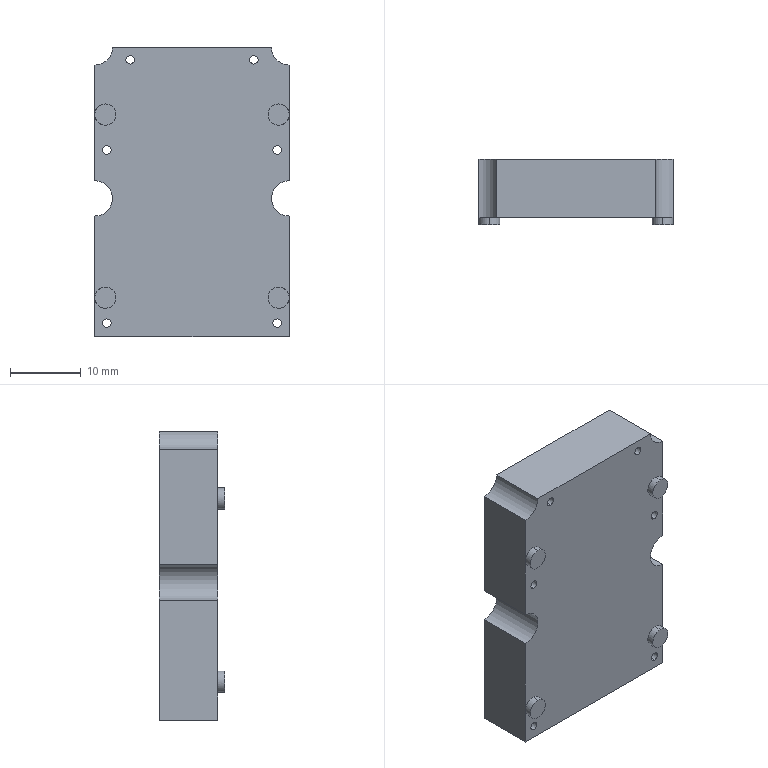Part | SolidWorks | features Extrusion 1, ICE 1, Scale 1 | 1 solid | 36 faces | box 27.5 x 9.25 x 40.9 mm | volume 9008 mm3 | cylinder 24 | plane 12 | commonest cylinder face diameters 1.2 x12 3 x8 5 x4
STEP:
#1=CARTESIAN_POINT('',(-12.25,3.11,-16.627));
#2=VERTEX_POINT('',#1);
#3=CARTESIAN_POINT('',(-12.25,3.11,-13.627));
#4=VERTEX_POINT('',#3);
#5=CARTESIAN_POINT('',(-12.25,3.11,-15.127));
#6=DIRECTION('',(0.,-1.,0.));
#7=DIRECTION('',(0.,0.,-1.));
#8=AXIS2_PLACEMENT_3D('',#5,#6,#7);
#9=CIRCLE('',#8,1.5);
#10=EDGE_CURVE('',#2,#4,#9,.T.);
#11=ORIENTED_EDGE('',*,*,#10,.F.);
#12=CARTESIAN_POINT('',(-12.25,4.11,-16.627));
#13=VERTEX_POINT('',#12);
#14=CARTESIAN_POINT('',(-12.25,3.11,-16.627));
#15=DIRECTION('',(0.,1.,0.));
#16=VECTOR('',#15,1000.);
#17=LINE('',#14,#16);
#18=EDGE_CURVE('',#2,#13,#17,.T.);
#19=ORIENTED_EDGE('',*,*,#18,.T.);
#20=CARTESIAN_POINT('',(-12.25,4.11,-13.627));
#21=VERTEX_POINT('',#20);
#22=CARTESIAN_POINT('',(-12.25,4.11,-15.127));
#23=DIRECTION('',(0.,-1.,0.));
#24=DIRECTION('',(0.,0.,-1.));
#25=AXIS2_PLACEMENT_3D('',#22,#23,#24);
#26=CIRCLE('',#25,1.5);
#27=EDGE_CURVE('',#13,#21,#26,.T.);
#28=ORIENTED_EDGE('',*,*,#27,.T.);
#29=CARTESIAN_POINT('',(-12.25,3.11,-13.627));
#30=DIRECTION('',(0.,1.,0.));
#31=VECTOR('',#30,1000.);
#32=LINE('',#29,#31);
#33=EDGE_CURVE('',#4,#21,#32,.T.);
#34=ORIENTED_EDGE('',*,*,#33,.F.);
#35=EDGE_LOOP('',(#11,#19,#28,#34));
#36=FACE_OUTER_BOUND('',#35,.T.);
#37=CARTESIAN_POINT('',(-12.25,3.11,-15.127));
#38=DIRECTION('',(0.,1.,0.));
#39=DIRECTION('',(0.,0.,1.));
#40=AXIS2_PLACEMENT_3D('',#37,#38,#39);
#41=CYLINDRICAL_SURFACE('',#40,1.5);
#42=ADVANCED_FACE('',(#36),#41,.T.);
#43=CARTESIAN_POINT('',(-12.25,3.11,9.273));
#44=VERTEX_POINT('',#43);
#45=CARTESIAN_POINT('',(-12.25,3.11,12.273));
#46=VERTEX_POINT('',#45);
#47=CARTESIAN_POINT('',(-12.25,3.11,10.773));
#48=DIRECTION('',(0.,-1.,0.));
#49=DIRECTION('',(0.,0.,-1.));
#50=AXIS2_PLACEMENT_3D('',#47,#48,#49);
#51=CIRCLE('',#50,1.5);
#52=EDGE_CURVE('',#44,#46,#51,.T.);
#53=ORIENTED_EDGE('',*,*,#52,.F.);
#54=CARTESIAN_POINT('',(-12.25,4.11,9.273));
#55=VERTEX_POINT('',#54);
#56=CARTESIAN_POINT('',(-12.25,3.11,9.273));
#57=DIRECTION('',(0.,1.,0.));
#58=VECTOR('',#57,1000.);
#59=LINE('',#56,#58);
#60=EDGE_CURVE('',#44,#55,#59,.T.);
#61=ORIENTED_EDGE('',*,*,#60,.T.);
#62=CARTESIAN_POINT('',(-12.25,4.11,12.273));
#63=VERTEX_POINT('',#62);
#64=CARTESIAN_POINT('',(-12.25,4.11,10.773));
#65=DIRECTION('',(0.,-1.,0.));
#66=DIRECTION('',(0.,0.,-1.));
#67=AXIS2_PLACEMENT_3D('',#64,#65,#66);
#68=CIRCLE('',#67,1.5);
#69=EDGE_CURVE('',#55,#63,#68,.T.);
#70=ORIENTED_EDGE('',*,*,#69,.T.);
#71=CARTESIAN_POINT('',(-12.25,3.11,12.273));
#72=DIRECTION('',(0.,1.,0.));
#73=VECTOR('',#72,1000.);
#74=LINE('',#71,#73);
#75=EDGE_CURVE('',#46,#63,#74,.T.);
#76=ORIENTED_EDGE('',*,*,#75,.F.);
#77=EDGE_LOOP('',(#53,#61,#70,#76));
#78=FACE_OUTER_BOUND('',#77,.T.);
#79=CARTESIAN_POINT('',(-12.25,3.11,10.773));
#80=DIRECTION('',(0.,1.,0.));
#81=DIRECTION('',(0.,0.,1.));
#82=AXIS2_PLACEMENT_3D('',#79,#80,#81);
#83=CYLINDRICAL_SURFACE('',#82,1.5);
#84=ADVANCED_FACE('',(#78),#83,.T.);
#85=CARTESIAN_POINT('',(12.25,3.11,9.273));
#86=VERTEX_POINT('',#85);
#87=CARTESIAN_POINT('',(12.25,3.11,12.273));
#88=VERTEX_POINT('',#87);
#89=CARTESIAN_POINT('',(12.25,3.11,10.773));
#90=DIRECTION('',(0.,-1.,0.));
#91=DIRECTION('',(0.,0.,-1.));
#92=AXIS2_PLACEMENT_3D('',#89,#90,#91);
#93=CIRCLE('',#92,1.5);
#94=EDGE_CURVE('',#86,#88,#93,.T.);
#95=ORIENTED_EDGE('',*,*,#94,.F.);
#96=CARTESIAN_POINT('',(12.25,4.11,9.273));
#97=VERTEX_POINT('',#96);
#98=CARTESIAN_POINT('',(12.25,3.11,9.273));
#99=DIRECTION('',(0.,1.,0.));
#100=VECTOR('',#99,1000.);
#101=LINE('',#98,#100);
#102=EDGE_CURVE('',#86,#97,#101,.T.);
#103=ORIENTED_EDGE('',*,*,#102,.T.);
#104=CARTESIAN_POINT('',(13.75,4.11,10.773));
#105=VERTEX_POINT('',#104);
#106=CARTESIAN_POINT('',(12.25,4.11,10.773));
#107=DIRECTION('',(0.,-1.,0.));
#108=DIRECTION('',(0.,0.,-1.));
#109=AXIS2_PLACEMENT_3D('',#106,#107,#108);
#110=CIRCLE('',#109,1.5);
#111=EDGE_CURVE('',#97,#105,#110,.T.);
#112=ORIENTED_EDGE('',*,*,#111,.T.);
#113=CARTESIAN_POINT('',(12.25,4.11,12.273));
#114=VERTEX_POINT('',#113);
#115=CARTESIAN_POINT('',(12.25,4.11,10.773));
#116=DIRECTION('',(0.,-1.,0.));
#117=DIRECTION('',(0.,0.,-1.));
#118=AXIS2_PLACEMENT_3D('',#115,#116,#117);
#119=CIRCLE('',#118,1.5);
#120=EDGE_CURVE('',#105,#114,#119,.T.);
#121=ORIENTED_EDGE('',*,*,#120,.T.);
#122=CARTESIAN_POINT('',(12.25,3.11,12.273));
#123=DIRECTION('',(0.,1.,0.));
#124=VECTOR('',#123,1000.);
#125=LINE('',#122,#124);
#126=EDGE_CURVE('',#88,#114,#125,.T.);
#127=ORIENTED_EDGE('',*,*,#126,.F.);
#128=EDGE_LOOP('',(#95,#103,#112,#121,#127));
#129=FACE_OUTER_BOUND('',#128,.T.);
#130=CARTESIAN_POINT('',(12.25,3.11,10.773));
#131=DIRECTION('',(0.,1.,0.));
#132=DIRECTION('',(0.,0.,1.));
#133=AXIS2_PLACEMENT_3D('',#130,#131,#132);
#134=CYLINDRICAL_SURFACE('',#133,1.5);
#135=ADVANCED_FACE('',(#129),#134,.T.);
#136=CARTESIAN_POINT('',(12.25,3.11,-16.627));
#137=VERTEX_POINT('',#136);
#138=CARTESIAN_POINT('',(12.25,3.11,-13.627));
#139=VERTEX_POINT('',#138);
#140=CARTESIAN_POINT('',(12.25,3.11,-15.127));
#141=DIRECTION('',(0.,-1.,0.));
#142=DIRECTION('',(0.,0.,-1.));
#143=AXIS2_PLACEMENT_3D('',#140,#141,#142);
#144=CIRCLE('',#143,1.5);
#145=EDGE_CURVE('',#137,#139,#144,.T.);
#146=ORIENTED_EDGE('',*,*,#145,.F.);
#147=CARTESIAN_POINT('',(12.25,4.11,-16.627));
#148=VERTEX_POINT('',#147);
#149=CARTESIAN_POINT('',(12.25,3.11,-16.627));
#150=DIRECTION('',(0.,1.,0.));
#151=VECTOR('',#150,1000.);
#152=LINE('',#149,#151);
#153=EDGE_CURVE('',#137,#148,#152,.T.);
#154=ORIENTED_EDGE('',*,*,#153,.T.);
#155=CARTESIAN_POINT('',(13.75,4.11,-15.127));
#156=VERTEX_POINT('',#155);
#157=CARTESIAN_POINT('',(12.25,4.11,-15.127));
#158=DIRECTION('',(0.,-1.,0.));
#159=DIRECTION('',(0.,0.,-1.));
#160=AXIS2_PLACEMENT_3D('',#157,#158,#159);
#161=CIRCLE('',#160,1.5);
#162=EDGE_CURVE('',#148,#156,#161,.T.);
#163=ORIENTED_EDGE('',*,*,#162,.T.);
#164=CARTESIAN_POINT('',(12.25,4.11,-13.627));
#165=VERTEX_POINT('',#164);
#166=CARTESIAN_POINT('',(12.25,4.11,-15.127));
#167=DIRECTION('',(0.,-1.,0.));
#168=DIRECTION('',(0.,0.,-1.));
#169=AXIS2_PLACEMENT_3D('',#166,#167,#168);
#170=CIRCLE('',#169,1.5);
#171=EDGE_CURVE('',#156,#165,#170,.T.);
#172=ORIENTED_EDGE('',*,*,#171,.T.);
#173=CARTESIAN_POINT('',(12.25,3.11,-13.627));
#174=DIRECTION('',(0.,1.,0.));
#175=VECTOR('',#174,1000.);
#176=LINE('',#173,#175);
#177=EDGE_CURVE('',#139,#165,#176,.T.);
#178=ORIENTED_EDGE('',*,*,#177,.F.);
#179=EDGE_LOOP('',(#146,#154,#163,#172,#178));
#180=FACE_OUTER_BOUND('',#179,.T.);
#181=CARTESIAN_POINT('',(12.25,3.11,-15.127));
#182=DIRECTION('',(0.,1.,0.));
#183=DIRECTION('',(0.,0.,1.));
#184=AXIS2_PLACEMENT_3D('',#181,#182,#183);
#185=CYLINDRICAL_SURFACE('',#184,1.5);
#186=ADVANCED_FACE('',(#180),#185,.T.);
#187=CARTESIAN_POINT('',(12.05,12.36,-19.327));
#188=VERTEX_POINT('',#187);
#189=CARTESIAN_POINT('',(12.05,12.36,-18.127));
#190=VERTEX_POINT('',#189);
#191=CARTESIAN_POINT('',(12.05,12.36,-18.727));
#192=DIRECTION('',(0.,1.,0.));
#193=DIRECTION('',(0.,0.,-1.));
#194=AXIS2_PLACEMENT_3D('',#191,#192,#193);
#195=CIRCLE('',#194,0.6);
#196=EDGE_CURVE('',#188,#190,#195,.T.);
#197=ORIENTED_EDGE('',*,*,#196,.T.);
#198=CARTESIAN_POINT('',(12.05,4.11,-18.127));
#199=VERTEX_POINT('',#198);
#200=CARTESIAN_POINT('',(12.05,12.36,-18.127));
#201=DIRECTION('',(0.,-1.,0.));
#202=VECTOR('',#201,1000.);
#203=LINE('',#200,#202);
#204=EDGE_CURVE('',#190,#199,#203,.T.);
#205=ORIENTED_EDGE('',*,*,#204,.T.);
#206=CARTESIAN_POINT('',(12.05,4.11,-19.327));
#207=VERTEX_POINT('',#206);
#208=CARTESIAN_POINT('',(12.05,4.11,-18.727));
#209=DIRECTION('',(0.,1.,0.));
#210=DIRECTION('',(0.,0.,-1.));
#211=AXIS2_PLACEMENT_3D('',#208,#209,#210);
#212=CIRCLE('',#211,0.6);
#213=EDGE_CURVE('',#207,#199,#212,.T.);
#214=ORIENTED_EDGE('',*,*,#213,.F.);
#215=CARTESIAN_POINT('',(12.05,12.36,-19.327));
#216=DIRECTION('',(0.,-1.,0.));
#217=VECTOR('',#216,1000.);
#218=LINE('',#215,#217);
#219=EDGE_CURVE('',#188,#207,#218,.T.);
#220=ORIENTED_EDGE('',*,*,#219,.F.);
#221=EDGE_LOOP('',(#197,#205,#214,#220));
#222=FACE_OUTER_BOUND('',#221,.T.);
#223=CARTESIAN_POINT('',(12.05,12.36,-18.727));
#224=DIRECTION('',(0.,-1.,0.));
#225=DIRECTION('',(0.,0.,-1.));
#226=AXIS2_PLACEMENT_3D('',#223,#224,#225);
#227=CYLINDRICAL_SURFACE('',#226,0.6);
#228=ADVANCED_FACE('',(#222),#227,.F.);
#229=CARTESIAN_POINT('',(12.05,12.36,5.173));
#230=VERTEX_POINT('',#229);
#231=CARTESIAN_POINT('',(12.05,12.36,6.373));
#232=VERTEX_POINT('',#231);
#233=CARTESIAN_POINT('',(12.05,12.36,5.773));
#234=DIRECTION('',(0.,1.,0.));
#235=DIRECTION('',(0.,0.,-1.));
#236=AXIS2_PLACEMENT_3D('',#233,#234,#235);
#237=CIRCLE('',#236,0.6);
#238=EDGE_CURVE('',#230,#232,#237,.T.);
#239=ORIENTED_EDGE('',*,*,#238,.T.);
#240=CARTESIAN_POINT('',(12.05,4.11,6.373));
#241=VERTEX_POINT('',#240);
#242=CARTESIAN_POINT('',(12.05,12.36,6.373));
#243=DIRECTION('',(0.,-1.,0.));
#244=VECTOR('',#243,1000.);
#245=LINE('',#242,#244);
#246=EDGE_CURVE('',#232,#241,#245,.T.);
#247=ORIENTED_EDGE('',*,*,#246,.T.);
#248=CARTESIAN_POINT('',(12.05,4.11,5.173));
#249=VERTEX_POINT('',#248);
#250=CARTESIAN_POINT('',(12.05,4.11,5.773));
#251=DIRECTION('',(0.,1.,0.));
#252=DIRECTION('',(0.,0.,-1.));
#253=AXIS2_PLACEMENT_3D('',#250,#251,#252);
#254=CIRCLE('',#253,0.6);
#255=EDGE_CURVE('',#249,#241,#254,.T.);
#256=ORIENTED_EDGE('',*,*,#255,.F.);
#257=CARTESIAN_POINT('',(12.05,12.36,5.173));
#258=DIRECTION('',(0.,-1.,0.));
#259=VECTOR('',#258,1000.);
#260=LINE('',#257,#259);
#261=EDGE_CURVE('',#230,#249,#260,.T.);
#262=ORIENTED_EDGE('',*,*,#261,.F.);
#263=EDGE_LOOP('',(#239,#247,#256,#262));
#264=FACE_OUTER_BOUND('',#263,.T.);
#265=CARTESIAN_POINT('',(12.05,12.36,5.773));
#266=DIRECTION('',(0.,-1.,0.));
#267=DIRECTION('',(0.,0.,-1.));
#268=AXIS2_PLACEMENT_3D('',#265,#266,#267);
#269=CYLINDRICAL_SURFACE('',#268,0.6);
#270=ADVANCED_FACE('',(#264),#269,.F.);
#271=CARTESIAN_POINT('',(8.75,12.36,17.923));
#272=VERTEX_POINT('',#271);
#273=CARTESIAN_POINT('',(8.75,12.36,19.123));
#274=VERTEX_POINT('',#273);
#275=CARTESIAN_POINT('',(8.75,12.36,18.523));
#276=DIRECTION('',(0.,1.,0.));
#277=DIRECTION('',(0.,0.,-1.));
#278=AXIS2_PLACEMENT_3D('',#275,#276,#277);
#279=CIRCLE('',#278,0.6);
#280=EDGE_CURVE('',#272,#274,#279,.T.);
#281=ORIENTED_EDGE('',*,*,#280,.T.);
#282=CARTESIAN_POINT('',(8.75,4.11,19.123));
#283=VERTEX_POINT('',#282);
#284=CARTESIAN_POINT('',(8.75,12.36,19.123));
#285=DIRECTION('',(0.,-1.,0.));
#286=VECTOR('',#285,1000.);
#287=LINE('',#284,#286);
#288=EDGE_CURVE('',#274,#283,#287,.T.);
#289=ORIENTED_EDGE('',*,*,#288,.T.);
#290=CARTESIAN_POINT('',(8.75,4.11,17.923));
#291=VERTEX_POINT('',#290);
#292=CARTESIAN_POINT('',(8.75,4.11,18.523));
#293=DIRECTION('',(0.,1.,0.));
#294=DIRECTION('',(0.,0.,-1.));
#295=AXIS2_PLACEMENT_3D('',#292,#293,#294);
#296=CIRCLE('',#295,0.6);
#297=EDGE_CURVE('',#291,#283,#296,.T.);
#298=ORIENTED_EDGE('',*,*,#297,.F.);
#299=CARTESIAN_POINT('',(8.75,12.36,17.923));
#300=DIRECTION('',(0.,-1.,0.));
#301=VECTOR('',#300,1000.);
#302=LINE('',#299,#301);
#303=EDGE_CURVE('',#272,#291,#302,.T.);
#304=ORIENTED_EDGE('',*,*,#303,.F.);
#305=EDGE_LOOP('',(#281,#289,#298,#304));
#306=FACE_OUTER_BOUND('',#305,.T.);
#307=CARTESIAN_POINT('',(8.75,12.36,18.523));
#308=DIRECTION('',(0.,-1.,0.));
#309=DIRECTION('',(0.,0.,-1.));
#310=AXIS2_PLACEMENT_3D('',#307,#308,#309);
#311=CYLINDRICAL_SURFACE('',#310,0.6);
#312=ADVANCED_FACE('',(#306),#311,.F.);
#313=CARTESIAN_POINT('',(-8.75,12.36,17.923));
#314=VERTEX_POINT('',#313);
#315=CARTESIAN_POINT('',(-8.75,12.36,19.123));
#316=VERTEX_POINT('',#315);
#317=CARTESIAN_POINT('',(-8.75,12.36,18.523));
#318=DIRECTION('',(0.,1.,0.));
#319=DIRECTION('',(0.,0.,1.));
#320=AXIS2_PLACEMENT_3D('',#317,#318,#319);
#321=CIRCLE('',#320,0.6);
#322=EDGE_CURVE('',#314,#316,#321,.T.);
#323=ORIENTED_EDGE('',*,*,#322,.T.);
#324=CARTESIAN_POINT('',(-8.75,4.11,19.123));
#325=VERTEX_POINT('',#324);
#326=CARTESIAN_POINT('',(-8.75,12.36,19.123));
#327=DIRECTION('',(0.,-1.,0.));
#328=VECTOR('',#327,1000.);
#329=LINE('',#326,#328);
#330=EDGE_CURVE('',#316,#325,#329,.T.);
#331=ORIENTED_EDGE('',*,*,#330,.T.);
#332=CARTESIAN_POINT('',(-8.75,4.11,17.923));
#333=VERTEX_POINT('',#332);
#334=CARTESIAN_POINT('',(-8.75,4.11,18.523));
#335=DIRECTION('',(0.,1.,0.));
#336=DIRECTION('',(0.,0.,1.));
#337=AXIS2_PLACEMENT_3D('',#334,#335,#336);
#338=CIRCLE('',#337,0.6);
#339=EDGE_CURVE('',#333,#325,#338,.T.);
#340=ORIENTED_EDGE('',*,*,#339,.F.);
#341=CARTESIAN_POINT('',(-8.75,12.36,17.923));
#342=DIRECTION('',(0.,-1.,0.));
#343=VECTOR('',#342,1000.);
#344=LINE('',#341,#343);
#345=EDGE_CURVE('',#314,#333,#344,.T.);
#346=ORIENTED_EDGE('',*,*,#345,.F.);
#347=EDGE_LOOP('',(#323,#331,#340,#346));
#348=FACE_OUTER_BOUND('',#347,.T.);
#349=CARTESIAN_POINT('',(-8.75,12.36,18.523));
#350=DIRECTION('',(0.,-1.,0.));
#351=DIRECTION('',(0.,0.,-1.));
#352=AXIS2_PLACEMENT_3D('',#349,#350,#351);
#353=CYLINDRICAL_SURFACE('',#352,0.6);
#354=ADVANCED_FACE('',(#348),#353,.F.);
#355=CARTESIAN_POINT('',(-12.05,12.36,5.173));
#356=VERTEX_POINT('',#355);
#357=CARTESIAN_POINT('',(-12.05,12.36,6.373));
#358=VERTEX_POINT('',#357);
#359=CARTESIAN_POINT('',(-12.05,12.36,5.773));
#360=DIRECTION('',(0.,1.,0.));
#361=DIRECTION('',(0.,0.,1.));
#362=AXIS2_PLACEMENT_3D('',#359,#360,#361);
#363=CIRCLE('',#362,0.6);
#364=EDGE_CURVE('',#356,#358,#363,.T.);
#365=ORIENTED_EDGE('',*,*,#364,.T.);
#366=CARTESIAN_POINT('',(-12.05,4.11,6.373));
#367=VERTEX_POINT('',#366);
#368=CARTESIAN_POINT('',(-12.05,12.36,6.373));
#369=DIRECTION('',(0.,-1.,0.));
#370=VECTOR('',#369,1000.);
#371=LINE('',#368,#370);
#372=EDGE_CURVE('',#358,#367,#371,.T.);
#373=ORIENTED_EDGE('',*,*,#372,.T.);
#374=CARTESIAN_POINT('',(-12.05,4.11,5.173));
#375=VERTEX_POINT('',#374);
#376=CARTESIAN_POINT('',(-12.05,4.11,5.773));
#377=DIRECTION('',(0.,1.,0.));
#378=DIRECTION('',(0.,0.,1.));
#379=AXIS2_PLACEMENT_3D('',#376,#377,#378);
#380=CIRCLE('',#379,0.6);
#381=EDGE_CURVE('',#375,#367,#380,.T.);
#382=ORIENTED_EDGE('',*,*,#381,.F.);
#383=CARTESIAN_POINT('',(-12.05,12.36,5.173));
#384=DIRECTION('',(0.,-1.,0.));
#385=VECTOR('',#384,1000.);
#386=LINE('',#383,#385);
#387=EDGE_CURVE('',#356,#375,#386,.T.);
#388=ORIENTED_EDGE('',*,*,#387,.F.);
#389=EDGE_LOOP('',(#365,#373,#382,#388));
#390=FACE_OUTER_BOUND('',#389,.T.);
#391=CARTESIAN_POINT('',(-12.05,12.36,5.773));
#392=DIRECTION('',(0.,-1.,0.));
#393=DIRECTION('',(0.,0.,-1.));
#394=AXIS2_PLACEMENT_3D('',#391,#392,#393);
#395=CYLINDRICAL_SURFACE('',#394,0.6);
#396=ADVANCED_FACE('',(#390),#395,.F.);
#397=CARTESIAN_POINT('',(-12.05,12.36,-19.327));
#398=VERTEX_POINT('',#397);
#399=CARTESIAN_POINT('',(-12.05,12.36,-18.127));
#400=VERTEX_POINT('',#399);
#401=CARTESIAN_POINT('',(-12.05,12.36,-18.727));
#402=DIRECTION('',(0.,1.,0.));
#403=DIRECTION('',(0.,0.,1.));
#404=AXIS2_PLACEMENT_3D('',#401,#402,#403);
#405=CIRCLE('',#404,0.6);
#406=EDGE_CURVE('',#398,#400,#405,.T.);
#407=ORIENTED_EDGE('',*,*,#406,.T.);
#408=CARTESIAN_POINT('',(-12.05,4.11,-18.127));
#409=VERTEX_POINT('',#408);
#410=CARTESIAN_POINT('',(-12.05,12.36,-18.127));
#411=DIRECTION('',(0.,-1.,0.));
#412=VECTOR('',#411,1000.);
#413=LINE('',#410,#412);
#414=EDGE_CURVE('',#400,#409,#413,.T.);
#415=ORIENTED_EDGE('',*,*,#414,.T.);
#416=CARTESIAN_POINT('',(-12.05,4.11,-19.327));
#417=VERTEX_POINT('',#416);
#418=CARTESIAN_POINT('',(-12.05,4.11,-18.727));
#419=DIRECTION('',(0.,1.,0.));
#420=DIRECTION('',(0.,0.,1.));
#421=AXIS2_PLACEMENT_3D('',#418,#419,#420);
#422=CIRCLE('',#421,0.6);
#423=EDGE_CURVE('',#417,#409,#422,.T.);
#424=ORIENTED_EDGE('',*,*,#423,.F.);
#425=CARTESIAN_POINT('',(-12.05,12.36,-19.327));
#426=DIRECTION('',(0.,-1.,0.));
#427=VECTOR('',#426,1000.);
#428=LINE('',#425,#427);
#429=EDGE_CURVE('',#398,#417,#428,.T.);
#430=ORIENTED_EDGE('',*,*,#429,.F.);
#431=EDGE_LOOP('',(#407,#415,#424,#430));
#432=FACE_OUTER_BOUND('',#431,.T.);
#433=CARTESIAN_POINT('',(-12.05,12.36,-18.727));
#434=DIRECTION('',(0.,-1.,0.));
#435=DIRECTION('',(0.,0.,-1.));
#436=AXIS2_PLACEMENT_3D('',#433,#434,#435);
#437=CYLINDRICAL_SURFACE('',#436,0.6);
#438=ADVANCED_FACE('',(#432),#437,.F.);
#439=ORIENTED_EDGE('',*,*,#238,.F.);
#440=CARTESIAN_POINT('',(12.05,12.36,5.773));
#441=DIRECTION('',(0.,1.,0.));
#442=DIRECTION('',(0.,0.,-1.));
#443=AXIS2_PLACEMENT_3D('',#440,#441,#442);
#444=CIRCLE('',#443,0.6);
#445=EDGE_CURVE('',#232,#230,#444,.T.);
#446=ORIENTED_EDGE('',*,*,#445,.F.);
#447=EDGE_LOOP('',(#439,#446));
#448=FACE_BOUND('',#447,.T.);
#449=ORIENTED_EDGE('',*,*,#322,.F.);
#450=CARTESIAN_POINT('',(-8.75,12.36,18.523));
#451=DIRECTION('',(0.,1.,0.));
#452=DIRECTION('',(0.,0.,1.));
#453=AXIS2_PLACEMENT_3D('',#450,#451,#452);
#454=CIRCLE('',#453,0.6);
#455=EDGE_CURVE('',#316,#314,#454,.T.);
#456=ORIENTED_EDGE('',*,*,#455,.F.);
#457=EDGE_LOOP('',(#449,#456));
#458=FACE_BOUND('',#457,.T.);
#459=ORIENTED_EDGE('',*,*,#406,.F.);
#460=CARTESIAN_POINT('',(-12.05,12.36,-18.727));
#461=DIRECTION('',(0.,1.,0.));
#462=DIRECTION('',(0.,0.,1.));
#463=AXIS2_PLACEMENT_3D('',#460,#461,#462);
#464=CIRCLE('',#463,0.6);
#465=EDGE_CURVE('',#400,#398,#464,.T.);
#466=ORIENTED_EDGE('',*,*,#465,.F.);
#467=EDGE_LOOP('',(#459,#466));
#468=FACE_BOUND('',#467,.T.);
#469=CARTESIAN_POINT('',(13.75,12.36,-3.577));
#470=VERTEX_POINT('',#469);
#471=CARTESIAN_POINT('',(13.75,12.36,-20.627));
#472=VERTEX_POINT('',#471);
#473=CARTESIAN_POINT('',(13.75,12.36,-3.577));
#474=DIRECTION('',(0.,0.,-1.));
#475=VECTOR('',#474,1000.);
#476=LINE('',#473,#475);
#477=EDGE_CURVE('',#470,#472,#476,.T.);
#478=ORIENTED_EDGE('',*,*,#477,.T.);
#479=CARTESIAN_POINT('',(-13.75,12.36,-20.627));
#480=VERTEX_POINT('',#479);
#481=CARTESIAN_POINT('',(-13.75,12.36,-20.627));
#482=DIRECTION('',(-1.,0.,0.));
#483=VECTOR('',#482,1000.);
#484=LINE('',#481,#483);
#485=EDGE_CURVE('',#472,#480,#484,.T.);
#486=ORIENTED_EDGE('',*,*,#485,.T.);
#487=CARTESIAN_POINT('',(-13.75,12.36,-3.577));
#488=VERTEX_POINT('',#487);
#489=CARTESIAN_POINT('',(-13.75,12.36,-3.577));
#490=DIRECTION('',(0.,0.,1.));
#491=VECTOR('',#490,1000.);
#492=LINE('',#489,#491);
#493=EDGE_CURVE('',#480,#488,#492,.T.);
#494=ORIENTED_EDGE('',*,*,#493,.T.);
#495=CARTESIAN_POINT('',(-13.75,12.36,1.423));
#496=VERTEX_POINT('',#495);
#497=CARTESIAN_POINT('',(-13.75,12.36,-1.077));
#498=DIRECTION('',(0.,-1.,0.));
#499=DIRECTION('',(0.,0.,1.));
#500=AXIS2_PLACEMENT_3D('',#497,#498,#499);
#501=CIRCLE('',#500,2.5);
#502=EDGE_CURVE('',#488,#496,#501,.T.);
#503=ORIENTED_EDGE('',*,*,#502,.T.);
#504=CARTESIAN_POINT('',(-13.75,12.36,17.773));
#505=VERTEX_POINT('',#504);
#506=CARTESIAN_POINT('',(-13.75,12.36,17.773));
#507=DIRECTION('',(0.,0.,1.));
#508=VECTOR('',#507,1000.);
#509=LINE('',#506,#508);
#510=EDGE_CURVE('',#496,#505,#509,.T.);
#511=ORIENTED_EDGE('',*,*,#510,.T.);
#512=CARTESIAN_POINT('',(-11.25,12.36,20.273));
#513=VERTEX_POINT('',#512);
#514=CARTESIAN_POINT('',(-13.75,12.36,20.273));
#515=DIRECTION('',(0.,-1.,0.));
#516=DIRECTION('',(0.,0.,1.));
#517=AXIS2_PLACEMENT_3D('',#514,#515,#516);
#518=CIRCLE('',#517,2.5);
#519=EDGE_CURVE('',#505,#513,#518,.T.);
#520=ORIENTED_EDGE('',*,*,#519,.T.);
#521=CARTESIAN_POINT('',(11.25,12.36,20.273));
#522=VERTEX_POINT('',#521);
#523=CARTESIAN_POINT('',(-11.25,12.36,20.273));
#524=DIRECTION('',(1.,0.,0.));
#525=VECTOR('',#524,1000.);
#526=LINE('',#523,#525);
#527=EDGE_CURVE('',#513,#522,#526,.T.);
#528=ORIENTED_EDGE('',*,*,#527,.T.);
#529=CARTESIAN_POINT('',(13.75,12.36,17.773));
#530=VERTEX_POINT('',#529);
#531=CARTESIAN_POINT('',(13.75,12.36,20.273));
#532=DIRECTION('',(0.,-1.,0.));
#533=DIRECTION('',(0.,0.,1.));
#534=AXIS2_PLACEMENT_3D('',#531,#532,#533);
#535=CIRCLE('',#534,2.5);
#536=EDGE_CURVE('',#522,#530,#535,.T.);
#537=ORIENTED_EDGE('',*,*,#536,.T.);
#538=CARTESIAN_POINT('',(13.75,12.36,1.423));
#539=VERTEX_POINT('',#538);
#540=CARTESIAN_POINT('',(13.75,12.36,17.773));
#541=DIRECTION('',(0.,0.,-1.));
#542=VECTOR('',#541,1000.);
#543=LINE('',#540,#542);
#544=EDGE_CURVE('',#530,#539,#543,.T.);
#545=ORIENTED_EDGE('',*,*,#544,.T.);
#546=CARTESIAN_POINT('',(13.75,12.36,-1.077));
#547=DIRECTION('',(0.,-1.,0.));
#548=DIRECTION('',(0.,0.,-1.));
#549=AXIS2_PLACEMENT_3D('',#546,#547,#548);
#550=CIRCLE('',#549,2.5);
#551=EDGE_CURVE('',#539,#470,#550,.T.);
#552=ORIENTED_EDGE('',*,*,#551,.T.);
#553=EDGE_LOOP('',(#478,#486,#494,#503,#511,#520,#528,#537,#545,#552));
#554=FACE_OUTER_BOUND('',#553,.T.);
#555=ORIENTED_EDGE('',*,*,#364,.F.);
#556=CARTESIAN_POINT('',(-12.05,12.36,5.773));
#557=DIRECTION('',(0.,1.,0.));
#558=DIRECTION('',(0.,0.,1.));
#559=AXIS2_PLACEMENT_3D('',#556,#557,#558);
#560=CIRCLE('',#559,0.6);
#561=EDGE_CURVE('',#358,#356,#560,.T.);
#562=ORIENTED_EDGE('',*,*,#561,.F.);
#563=EDGE_LOOP('',(#555,#562));
#564=FACE_BOUND('',#563,.T.);
#565=ORIENTED_EDGE('',*,*,#280,.F.);
#566=CARTESIAN_POINT('',(8.75,12.36,18.523));
#567=DIRECTION('',(0.,1.,0.));
#568=DIRECTION('',(0.,0.,-1.));
#569=AXIS2_PLACEMENT_3D('',#566,#567,#568);
#570=CIRCLE('',#569,0.6);
#571=EDGE_CURVE('',#274,#272,#570,.T.);
#572=ORIENTED_EDGE('',*,*,#571,.F.);
#573=EDGE_LOOP('',(#565,#572));
#574=FACE_BOUND('',#573,.T.);
#575=ORIENTED_EDGE('',*,*,#196,.F.);
#576=CARTESIAN_POINT('',(12.05,12.36,-18.727));
#577=DIRECTION('',(0.,1.,0.));
#578=DIRECTION('',(0.,0.,-1.));
#579=AXIS2_PLACEMENT_3D('',#576,#577,#578);
#580=CIRCLE('',#579,0.6);
#581=EDGE_CURVE('',#190,#188,#580,.T.);
#582=ORIENTED_EDGE('',*,*,#581,.F.);
#583=EDGE_LOOP('',(#575,#582));
#584=FACE_BOUND('',#583,.T.);
#585=CARTESIAN_POINT('',(-13.75,12.36,-1.077));
#586=DIRECTION('',(0.,1.,0.));
#587=DIRECTION('',(0.,0.,1.));
#588=AXIS2_PLACEMENT_3D('',#585,#586,#587);
#589=PLANE('',#588);
#590=ADVANCED_FACE('',(#448,#458,#468,#554,#564,#574,#584),#589,.T.);
#591=CARTESIAN_POINT('',(-13.75,4.11,-15.127));
#592=VERTEX_POINT('',#591);
#593=CARTESIAN_POINT('',(-13.75,4.11,-3.577));
#594=VERTEX_POINT('',#593);
#595=CARTESIAN_POINT('',(-13.75,4.11,-3.577));
#596=DIRECTION('',(0.,0.,1.));
#597=VECTOR('',#596,1000.);
#598=LINE('',#595,#597);
#599=EDGE_CURVE('',#592,#594,#598,.T.);
#600=ORIENTED_EDGE('',*,*,#599,.F.);
#601=CARTESIAN_POINT('',(-12.25,4.11,-15.127));
#602=DIRECTION('',(0.,-1.,0.));
#603=DIRECTION('',(0.,0.,-1.));
#604=AXIS2_PLACEMENT_3D('',#601,#602,#603);
#605=CIRCLE('',#604,1.5);
#606=EDGE_CURVE('',#21,#592,#605,.T.);
#607=ORIENTED_EDGE('',*,*,#606,.F.);
#608=ORIENTED_EDGE('',*,*,#27,.F.);
#609=CARTESIAN_POINT('',(-12.25,4.11,-15.127));
#610=DIRECTION('',(0.,-1.,0.));
#611=DIRECTION('',(0.,0.,-1.));
#612=AXIS2_PLACEMENT_3D('',#609,#610,#611);
#613=CIRCLE('',#612,1.5);
#614=EDGE_CURVE('',#592,#13,#613,.T.);
#615=ORIENTED_EDGE('',*,*,#614,.F.);
#616=CARTESIAN_POINT('',(-13.75,4.11,-20.627));
#617=VERTEX_POINT('',#616);
#618=CARTESIAN_POINT('',(-13.75,4.11,-3.577));
#619=DIRECTION('',(0.,0.,1.));
#620=VECTOR('',#619,1000.);
#621=LINE('',#618,#620);
#622=EDGE_CURVE('',#617,#592,#621,.T.);
#623=ORIENTED_EDGE('',*,*,#622,.F.);
#624=CARTESIAN_POINT('',(13.75,4.11,-20.627));
#625=VERTEX_POINT('',#624);
#626=CARTESIAN_POINT('',(-13.75,4.11,-20.627));
#627=DIRECTION('',(-1.,0.,0.));
#628=VECTOR('',#627,1000.);
#629=LINE('',#626,#628);
#630=EDGE_CURVE('',#625,#617,#629,.T.);
#631=ORIENTED_EDGE('',*,*,#630,.F.);
#632=CARTESIAN_POINT('',(13.75,4.11,-3.577));
#633=DIRECTION('',(0.,0.,-1.));
#634=VECTOR('',#633,1000.);
#635=LINE('',#632,#634);
#636=EDGE_CURVE('',#156,#625,#635,.T.);
#637=ORIENTED_EDGE('',*,*,#636,.F.);
#638=ORIENTED_EDGE('',*,*,#162,.F.);
#639=CARTESIAN_POINT('',(12.25,4.11,-15.127));
#640=DIRECTION('',(0.,-1.,0.));
#641=DIRECTION('',(0.,0.,-1.));
#642=AXIS2_PLACEMENT_3D('',#639,#640,#641);
#643=CIRCLE('',#642,1.5);
#644=EDGE_CURVE('',#165,#148,#643,.T.);
#645=ORIENTED_EDGE('',*,*,#644,.F.);
#646=ORIENTED_EDGE('',*,*,#171,.F.);
#647=CARTESIAN_POINT('',(13.75,4.11,-3.577));
#648=VERTEX_POINT('',#647);
#649=CARTESIAN_POINT('',(13.75,4.11,-3.577));
#650=DIRECTION('',(0.,0.,-1.));
#651=VECTOR('',#650,1000.);
#652=LINE('',#649,#651);
#653=EDGE_CURVE('',#648,#156,#652,.T.);
#654=ORIENTED_EDGE('',*,*,#653,.F.);
#655=CARTESIAN_POINT('',(13.75,4.11,1.423));
#656=VERTEX_POINT('',#655);
#657=CARTESIAN_POINT('',(13.75,4.11,-1.077));
#658=DIRECTION('',(0.,-1.,0.));
#659=DIRECTION('',(0.,0.,-1.));
#660=AXIS2_PLACEMENT_3D('',#657,#658,#659);
#661=CIRCLE('',#660,2.5);
#662=EDGE_CURVE('',#656,#648,#661,.T.);
#663=ORIENTED_EDGE('',*,*,#662,.F.);
#664=CARTESIAN_POINT('',(13.75,4.11,17.773));
#665=DIRECTION('',(0.,0.,-1.));
#666=VECTOR('',#665,1000.);
#667=LINE('',#664,#666);
#668=EDGE_CURVE('',#105,#656,#667,.T.);
#669=ORIENTED_EDGE('',*,*,#668,.F.);
#670=ORIENTED_EDGE('',*,*,#111,.F.);
#671=CARTESIAN_POINT('',(12.25,4.11,10.773));
#672=DIRECTION('',(0.,-1.,0.));
#673=DIRECTION('',(0.,0.,-1.));
#674=AXIS2_PLACEMENT_3D('',#671,#672,#673);
#675=CIRCLE('',#674,1.5);
#676=EDGE_CURVE('',#114,#97,#675,.T.);
#677=ORIENTED_EDGE('',*,*,#676,.F.);
#678=ORIENTED_EDGE('',*,*,#120,.F.);
#679=CARTESIAN_POINT('',(13.75,4.11,17.773));
#680=VERTEX_POINT('',#679);
#681=CARTESIAN_POINT('',(13.75,4.11,17.773));
#682=DIRECTION('',(0.,0.,-1.));
#683=VECTOR('',#682,1000.);
#684=LINE('',#681,#683);
#685=EDGE_CURVE('',#680,#105,#684,.T.);
#686=ORIENTED_EDGE('',*,*,#685,.F.);
#687=CARTESIAN_POINT('',(11.25,4.11,20.273));
#688=VERTEX_POINT('',#687);
#689=CARTESIAN_POINT('',(13.75,4.11,20.273));
#690=DIRECTION('',(0.,-1.,0.));
#691=DIRECTION('',(0.,0.,1.));
#692=AXIS2_PLACEMENT_3D('',#689,#690,#691);
#693=CIRCLE('',#692,2.5);
#694=EDGE_CURVE('',#688,#680,#693,.T.);
#695=ORIENTED_EDGE('',*,*,#694,.F.);
#696=CARTESIAN_POINT('',(-11.25,4.11,20.273));
#697=VERTEX_POINT('',#696);
#698=CARTESIAN_POINT('',(-11.25,4.11,20.273));
#699=DIRECTION('',(1.,0.,0.));
#700=VECTOR('',#699,1000.);
#701=LINE('',#698,#700);
#702=EDGE_CURVE('',#697,#688,#701,.T.);
#703=ORIENTED_EDGE('',*,*,#702,.F.);
#704=CARTESIAN_POINT('',(-13.75,4.11,17.773));
#705=VERTEX_POINT('',#704);
#706=CARTESIAN_POINT('',(-13.75,4.11,20.273));
#707=DIRECTION('',(0.,-1.,0.));
#708=DIRECTION('',(0.,0.,1.));
#709=AXIS2_PLACEMENT_3D('',#706,#707,#708);
#710=CIRCLE('',#709,2.5);
#711=EDGE_CURVE('',#705,#697,#710,.T.);
#712=ORIENTED_EDGE('',*,*,#711,.F.);
#713=CARTESIAN_POINT('',(-13.75,4.11,10.773));
#714=VERTEX_POINT('',#713);
#715=CARTESIAN_POINT('',(-13.75,4.11,17.773));
#716=DIRECTION('',(0.,0.,1.));
#717=VECTOR('',#716,1000.);
#718=LINE('',#715,#717);
#719=EDGE_CURVE('',#714,#705,#718,.T.);
#720=ORIENTED_EDGE('',*,*,#719,.F.);
#721=CARTESIAN_POINT('',(-12.25,4.11,10.773));
#722=DIRECTION('',(0.,-1.,0.));
#723=DIRECTION('',(0.,0.,-1.));
#724=AXIS2_PLACEMENT_3D('',#721,#722,#723);
#725=CIRCLE('',#724,1.5);
#726=EDGE_CURVE('',#63,#714,#725,.T.);
#727=ORIENTED_EDGE('',*,*,#726,.F.);
#728=ORIENTED_EDGE('',*,*,#69,.F.);
#729=CARTESIAN_POINT('',(-12.25,4.11,10.773));
#730=DIRECTION('',(0.,-1.,0.));
#731=DIRECTION('',(0.,0.,-1.));
#732=AXIS2_PLACEMENT_3D('',#729,#730,#731);
#733=CIRCLE('',#732,1.5);
#734=EDGE_CURVE('',#714,#55,#733,.T.);
#735=ORIENTED_EDGE('',*,*,#734,.F.);
#736=CARTESIAN_POINT('',(-13.75,4.11,1.423));
#737=VERTEX_POINT('',#736);
#738=CARTESIAN_POINT('',(-13.75,4.11,17.773));
#739=DIRECTION('',(0.,0.,1.));
#740=VECTOR('',#739,1000.);
#741=LINE('',#738,#740);
#742=EDGE_CURVE('',#737,#714,#741,.T.);
#743=ORIENTED_EDGE('',*,*,#742,.F.);
#744=CARTESIAN_POINT('',(-13.75,4.11,-1.077));
#745=DIRECTION('',(0.,-1.,0.));
#746=DIRECTION('',(0.,0.,1.));
#747=AXIS2_PLACEMENT_3D('',#744,#745,#746);
#748=CIRCLE('',#747,2.5);
#749=EDGE_CURVE('',#594,#737,#748,.T.);
#750=ORIENTED_EDGE('',*,*,#749,.F.);
#751=EDGE_LOOP('',(#600,#607,#608,#615,#623,#631,#637,#638,#645,#646,#654,#663,#669,#670,#677,#678,#686,#695,#703,#712,#720,#727,#728,#735,#743,#750));
#752=FACE_OUTER_BOUND('',#751,.T.);
#753=ORIENTED_EDGE('',*,*,#423,.T.);
#754=CARTESIAN_POINT('',(-12.05,4.11,-18.727));
#755=DIRECTION('',(0.,1.,0.));
#756=DIRECTION('',(0.,0.,1.));
#757=AXIS2_PLACEMENT_3D('',#754,#755,#756);
#758=CIRCLE('',#757,0.6);
#759=EDGE_CURVE('',#409,#417,#758,.T.);
#760=ORIENTED_EDGE('',*,*,#759,.T.);
#761=EDGE_LOOP('',(#753,#760));
#762=FACE_BOUND('',#761,.T.);
#763=ORIENTED_EDGE('',*,*,#381,.T.);
#764=CARTESIAN_POINT('',(-12.05,4.11,5.773));
#765=DIRECTION('',(0.,1.,0.));
#766=DIRECTION('',(0.,0.,1.));
#767=AXIS2_PLACEMENT_3D('',#764,#765,#766);
#768=CIRCLE('',#767,0.6);
#769=EDGE_CURVE('',#367,#375,#768,.T.);
#770=ORIENTED_EDGE('',*,*,#769,.T.);
#771=EDGE_LOOP('',(#763,#770));
#772=FACE_BOUND('',#771,.T.);
#773=ORIENTED_EDGE('',*,*,#339,.T.);
#774=CARTESIAN_POINT('',(-8.75,4.11,18.523));
#775=DIRECTION('',(0.,1.,0.));
#776=DIRECTION('',(0.,0.,1.));
#777=AXIS2_PLACEMENT_3D('',#774,#775,#776);
#778=CIRCLE('',#777,0.6);
#779=EDGE_CURVE('',#325,#333,#778,.T.);
#780=ORIENTED_EDGE('',*,*,#779,.T.);
#781=EDGE_LOOP('',(#773,#780));
#782=FACE_BOUND('',#781,.T.);
#783=ORIENTED_EDGE('',*,*,#297,.T.);
#784=CARTESIAN_POINT('',(8.75,4.11,18.523));
#785=DIRECTION('',(0.,1.,0.));
#786=DIRECTION('',(0.,0.,-1.));
#787=AXIS2_PLACEMENT_3D('',#784,#785,#786);
#788=CIRCLE('',#787,0.6);
#789=EDGE_CURVE('',#283,#291,#788,.T.);
#790=ORIENTED_EDGE('',*,*,#789,.T.);
#791=EDGE_LOOP('',(#783,#790));
#792=FACE_BOUND('',#791,.T.);
#793=ORIENTED_EDGE('',*,*,#255,.T.);
#794=CARTESIAN_POINT('',(12.05,4.11,5.773));
#795=DIRECTION('',(0.,1.,0.));
#796=DIRECTION('',(0.,0.,-1.));
#797=AXIS2_PLACEMENT_3D('',#794,#795,#796);
#798=CIRCLE('',#797,0.6);
#799=EDGE_CURVE('',#241,#249,#798,.T.);
#800=ORIENTED_EDGE('',*,*,#799,.T.);
#801=EDGE_LOOP('',(#793,#800));
#802=FACE_BOUND('',#801,.T.);
#803=ORIENTED_EDGE('',*,*,#213,.T.);
#804=CARTESIAN_POINT('',(12.05,4.11,-18.727));
#805=DIRECTION('',(0.,1.,0.));
#806=DIRECTION('',(0.,0.,-1.));
#807=AXIS2_PLACEMENT_3D('',#804,#805,#806);
#808=CIRCLE('',#807,0.6);
#809=EDGE_CURVE('',#199,#207,#808,.T.);
#810=ORIENTED_EDGE('',*,*,#809,.T.);
#811=EDGE_LOOP('',(#803,#810));
#812=FACE_BOUND('',#811,.T.);
#813=CARTESIAN_POINT('',(-13.75,4.11,-1.077));
#814=DIRECTION('',(0.,1.,0.));
#815=DIRECTION('',(0.,0.,1.));
#816=AXIS2_PLACEMENT_3D('',#813,#814,#815);
#817=PLANE('',#816);
#818=ADVANCED_FACE('',(#752,#762,#772,#782,#792,#802,#812),#817,.F.);
#819=ORIENTED_EDGE('',*,*,#653,.T.);
#820=ORIENTED_EDGE('',*,*,#636,.T.);
#821=CARTESIAN_POINT('',(13.75,12.36,-20.627));
#822=DIRECTION('',(0.,-1.,0.));
#823=VECTOR('',#822,1000.);
#824=LINE('',#821,#823);
#825=EDGE_CURVE('',#472,#625,#824,.T.);
#826=ORIENTED_EDGE('',*,*,#825,.F.);
#827=ORIENTED_EDGE('',*,*,#477,.F.);
#828=CARTESIAN_POINT('',(13.75,12.36,-3.577));
#829=DIRECTION('',(0.,-1.,0.));
#830=VECTOR('',#829,1000.);
#831=LINE('',#828,#830);
#832=EDGE_CURVE('',#470,#648,#831,.T.);
#833=ORIENTED_EDGE('',*,*,#832,.T.);
#834=EDGE_LOOP('',(#819,#820,#826,#827,#833));
#835=FACE_OUTER_BOUND('',#834,.T.);
#836=CARTESIAN_POINT('',(13.75,12.36,-3.577));
#837=DIRECTION('',(-1.,0.,0.));
#838=DIRECTION('',(0.,0.,1.));
#839=AXIS2_PLACEMENT_3D('',#836,#837,#838);
#840=PLANE('',#839);
#841=ADVANCED_FACE('',(#835),#840,.F.);
#842=ORIENTED_EDGE('',*,*,#630,.T.);
#843=CARTESIAN_POINT('',(-13.75,12.36,-20.627));
#844=DIRECTION('',(0.,-1.,0.));
#845=VECTOR('',#844,1000.);
#846=LINE('',#843,#845);
#847=EDGE_CURVE('',#480,#617,#846,.T.);
#848=ORIENTED_EDGE('',*,*,#847,.F.);
#849=ORIENTED_EDGE('',*,*,#485,.F.);
#850=ORIENTED_EDGE('',*,*,#825,.T.);
#851=EDGE_LOOP('',(#842,#848,#849,#850));
#852=FACE_OUTER_BOUND('',#851,.T.);
#853=CARTESIAN_POINT('',(-13.75,12.36,-20.627));
#854=DIRECTION('',(0.,0.,1.));
#855=DIRECTION('',(1.,0.,0.));
#856=AXIS2_PLACEMENT_3D('',#853,#854,#855);
#857=PLANE('',#856);
#858=ADVANCED_FACE('',(#852),#857,.F.);
#859=ORIENTED_EDGE('',*,*,#622,.T.);
#860=ORIENTED_EDGE('',*,*,#599,.T.);
#861=CARTESIAN_POINT('',(-13.75,12.36,-3.577));
#862=DIRECTION('',(0.,-1.,0.));
#863=VECTOR('',#862,1000.);
#864=LINE('',#861,#863);
#865=EDGE_CURVE('',#488,#594,#864,.T.);
#866=ORIENTED_EDGE('',*,*,#865,.F.);
#867=ORIENTED_EDGE('',*,*,#493,.F.);
#868=ORIENTED_EDGE('',*,*,#847,.T.);
#869=EDGE_LOOP('',(#859,#860,#866,#867,#868));
#870=FACE_OUTER_BOUND('',#869,.T.);
#871=CARTESIAN_POINT('',(-13.75,12.36,-3.577));
#872=DIRECTION('',(1.,0.,0.));
#873=DIRECTION('',(0.,0.,-1.));
#874=AXIS2_PLACEMENT_3D('',#871,#872,#873);
#875=PLANE('',#874);
#876=ADVANCED_FACE('',(#870),#875,.F.);
#877=ORIENTED_EDGE('',*,*,#749,.T.);
#878=CARTESIAN_POINT('',(-13.75,12.36,1.423));
#879=DIRECTION('',(0.,-1.,0.));
#880=VECTOR('',#879,1000.);
#881=LINE('',#878,#880);
#882=EDGE_CURVE('',#496,#737,#881,.T.);
#883=ORIENTED_EDGE('',*,*,#882,.F.);
#884=ORIENTED_EDGE('',*,*,#502,.F.);
#885=ORIENTED_EDGE('',*,*,#865,.T.);
#886=EDGE_LOOP('',(#877,#883,#884,#885));
#887=FACE_OUTER_BOUND('',#886,.T.);
#888=CARTESIAN_POINT('',(-13.75,12.36,-1.077));
#889=DIRECTION('',(0.,-1.,0.));
#890=DIRECTION('',(0.,0.,-1.));
#891=AXIS2_PLACEMENT_3D('',#888,#889,#890);
#892=CYLINDRICAL_SURFACE('',#891,2.5);
#893=ADVANCED_FACE('',(#887),#892,.F.);
#894=ORIENTED_EDGE('',*,*,#742,.T.);
#895=ORIENTED_EDGE('',*,*,#719,.T.);
#896=CARTESIAN_POINT('',(-13.75,12.36,17.773));
#897=DIRECTION('',(0.,-1.,0.));
#898=VECTOR('',#897,1000.);
#899=LINE('',#896,#898);
#900=EDGE_CURVE('',#505,#705,#899,.T.);
#901=ORIENTED_EDGE('',*,*,#900,.F.);
#902=ORIENTED_EDGE('',*,*,#510,.F.);
#903=ORIENTED_EDGE('',*,*,#882,.T.);
#904=EDGE_LOOP('',(#894,#895,#901,#902,#903));
#905=FACE_OUTER_BOUND('',#904,.T.);
#906=CARTESIAN_POINT('',(-13.75,12.36,17.773));
#907=DIRECTION('',(1.,0.,0.));
#908=DIRECTION('',(0.,0.,-1.));
#909=AXIS2_PLACEMENT_3D('',#906,#907,#908);
#910=PLANE('',#909);
#911=ADVANCED_FACE('',(#905),#910,.F.);
#912=ORIENTED_EDGE('',*,*,#711,.T.);
#913=CARTESIAN_POINT('',(-11.25,12.36,20.273));
#914=DIRECTION('',(0.,-1.,0.));
#915=VECTOR('',#914,1000.);
#916=LINE('',#913,#915);
#917=EDGE_CURVE('',#513,#697,#916,.T.);
#918=ORIENTED_EDGE('',*,*,#917,.F.);
#919=ORIENTED_EDGE('',*,*,#519,.F.);
#920=ORIENTED_EDGE('',*,*,#900,.T.);
#921=EDGE_LOOP('',(#912,#918,#919,#920));
#922=FACE_OUTER_BOUND('',#921,.T.);
#923=CARTESIAN_POINT('',(-13.75,12.36,20.273));
#924=DIRECTION('',(0.,-1.,0.));
#925=DIRECTION('',(0.,0.,-1.));
#926=AXIS2_PLACEMENT_3D('',#923,#924,#925);
#927=CYLINDRICAL_SURFACE('',#926,2.5);
#928=ADVANCED_FACE('',(#922),#927,.F.);
#929=ORIENTED_EDGE('',*,*,#702,.T.);
#930=CARTESIAN_POINT('',(11.25,12.36,20.273));
#931=DIRECTION('',(0.,-1.,0.));
#932=VECTOR('',#931,1000.);
#933=LINE('',#930,#932);
#934=EDGE_CURVE('',#522,#688,#933,.T.);
#935=ORIENTED_EDGE('',*,*,#934,.F.);
#936=ORIENTED_EDGE('',*,*,#527,.F.);
#937=ORIENTED_EDGE('',*,*,#917,.T.);
#938=EDGE_LOOP('',(#929,#935,#936,#937));
#939=FACE_OUTER_BOUND('',#938,.T.);
#940=CARTESIAN_POINT('',(-11.25,12.36,20.273));
#941=DIRECTION('',(0.,0.,-1.));
#942=DIRECTION('',(-1.,0.,0.));
#943=AXIS2_PLACEMENT_3D('',#940,#941,#942);
#944=PLANE('',#943);
#945=ADVANCED_FACE('',(#939),#944,.F.);
#946=ORIENTED_EDGE('',*,*,#694,.T.);
#947=CARTESIAN_POINT('',(13.75,12.36,17.773));
#948=DIRECTION('',(0.,-1.,0.));
#949=VECTOR('',#948,1000.);
#950=LINE('',#947,#949);
#951=EDGE_CURVE('',#530,#680,#950,.T.);
#952=ORIENTED_EDGE('',*,*,#951,.F.);
#953=ORIENTED_EDGE('',*,*,#536,.F.);
#954=ORIENTED_EDGE('',*,*,#934,.T.);
#955=EDGE_LOOP('',(#946,#952,#953,#954));
#956=FACE_OUTER_BOUND('',#955,.T.);
#957=CARTESIAN_POINT('',(13.75,12.36,20.273));
#958=DIRECTION('',(0.,-1.,0.));
#959=DIRECTION('',(0.,0.,-1.));
#960=AXIS2_PLACEMENT_3D('',#957,#958,#959);
#961=CYLINDRICAL_SURFACE('',#960,2.5);
#962=ADVANCED_FACE('',(#956),#961,.F.);
#963=ORIENTED_EDGE('',*,*,#685,.T.);
#964=ORIENTED_EDGE('',*,*,#668,.T.);
#965=CARTESIAN_POINT('',(13.75,12.36,1.423));
#966=DIRECTION('',(0.,-1.,0.));
#967=VECTOR('',#966,1000.);
#968=LINE('',#965,#967);
#969=EDGE_CURVE('',#539,#656,#968,.T.);
#970=ORIENTED_EDGE('',*,*,#969,.F.);
#971=ORIENTED_EDGE('',*,*,#544,.F.);
#972=ORIENTED_EDGE('',*,*,#951,.T.);
#973=EDGE_LOOP('',(#963,#964,#970,#971,#972));
#974=FACE_OUTER_BOUND('',#973,.T.);
#975=CARTESIAN_POINT('',(13.75,12.36,17.773));
#976=DIRECTION('',(-1.,0.,0.));
#977=DIRECTION('',(0.,0.,1.));
#978=AXIS2_PLACEMENT_3D('',#975,#976,#977);
#979=PLANE('',#978);
#980=ADVANCED_FACE('',(#974),#979,.F.);
#981=ORIENTED_EDGE('',*,*,#662,.T.);
#982=ORIENTED_EDGE('',*,*,#832,.F.);
#983=ORIENTED_EDGE('',*,*,#551,.F.);
#984=ORIENTED_EDGE('',*,*,#969,.T.);
#985=EDGE_LOOP('',(#981,#982,#983,#984));
#986=FACE_OUTER_BOUND('',#985,.T.);
#987=CARTESIAN_POINT('',(13.75,12.36,-1.077));
#988=DIRECTION('',(0.,-1.,0.));
#989=DIRECTION('',(0.,0.,-1.));
#990=AXIS2_PLACEMENT_3D('',#987,#988,#989);
#991=CYLINDRICAL_SURFACE('',#990,2.5);
#992=ADVANCED_FACE('',(#986),#991,.F.);
#993=ORIENTED_EDGE('',*,*,#414,.F.);
#994=ORIENTED_EDGE('',*,*,#465,.T.);
#995=ORIENTED_EDGE('',*,*,#429,.T.);
#996=ORIENTED_EDGE('',*,*,#759,.F.);
#997=EDGE_LOOP('',(#993,#994,#995,#996));
#998=FACE_OUTER_BOUND('',#997,.T.);
#999=CARTESIAN_POINT('',(-12.05,12.36,-18.727));
#1000=DIRECTION('',(0.,-1.,0.));
#1001=DIRECTION('',(0.,0.,-1.));
#1002=AXIS2_PLACEMENT_3D('',#999,#1000,#1001);
#1003=CYLINDRICAL_SURFACE('',#1002,0.6);
#1004=ADVANCED_FACE('',(#998),#1003,.F.);
#1005=ORIENTED_EDGE('',*,*,#372,.F.);
#1006=ORIENTED_EDGE('',*,*,#561,.T.);
#1007=ORIENTED_EDGE('',*,*,#387,.T.);
#1008=ORIENTED_EDGE('',*,*,#769,.F.);
#1009=EDGE_LOOP('',(#1005,#1006,#1007,#1008));
#1010=FACE_OUTER_BOUND('',#1009,.T.);
#1011=CARTESIAN_POINT('',(-12.05,12.36,5.773));
#1012=DIRECTION('',(0.,-1.,0.));
#1013=DIRECTION('',(0.,0.,-1.));
#1014=AXIS2_PLACEMENT_3D('',#1011,#1012,#1013);
#1015=CYLINDRICAL_SURFACE('',#1014,0.6);
#1016=ADVANCED_FACE('',(#1010),#1015,.F.);
#1017=ORIENTED_EDGE('',*,*,#330,.F.);
#1018=ORIENTED_EDGE('',*,*,#455,.T.);
#1019=ORIENTED_EDGE('',*,*,#345,.T.);
#1020=ORIENTED_EDGE('',*,*,#779,.F.);
#1021=EDGE_LOOP('',(#1017,#1018,#1019,#1020));
#1022=FACE_OUTER_BOUND('',#1021,.T.);
#1023=CARTESIAN_POINT('',(-8.75,12.36,18.523));
#1024=DIRECTION('',(0.,-1.,0.));
#1025=DIRECTION('',(0.,0.,-1.));
#1026=AXIS2_PLACEMENT_3D('',#1023,#1024,#1025);
#1027=CYLINDRICAL_SURFACE('',#1026,0.6);
#1028=ADVANCED_FACE('',(#1022),#1027,.F.);
#1029=ORIENTED_EDGE('',*,*,#288,.F.);
#1030=ORIENTED_EDGE('',*,*,#571,.T.);
#1031=ORIENTED_EDGE('',*,*,#303,.T.);
#1032=ORIENTED_EDGE('',*,*,#789,.F.);
#1033=EDGE_LOOP('',(#1029,#1030,#1031,#1032));
#1034=FACE_OUTER_BOUND('',#1033,.T.);
#1035=CARTESIAN_POINT('',(8.75,12.36,18.523));
#1036=DIRECTION('',(0.,-1.,0.));
#1037=DIRECTION('',(0.,0.,-1.));
#1038=AXIS2_PLACEMENT_3D('',#1035,#1036,#1037);
#1039=CYLINDRICAL_SURFACE('',#1038,0.6);
#1040=ADVANCED_FACE('',(#1034),#1039,.F.);
#1041=ORIENTED_EDGE('',*,*,#246,.F.);
#1042=ORIENTED_EDGE('',*,*,#445,.T.);
#1043=ORIENTED_EDGE('',*,*,#261,.T.);
#1044=ORIENTED_EDGE('',*,*,#799,.F.);
#1045=EDGE_LOOP('',(#1041,#1042,#1043,#1044));
#1046=FACE_OUTER_BOUND('',#1045,.T.);
#1047=CARTESIAN_POINT('',(12.05,12.36,5.773));
#1048=DIRECTION('',(0.,-1.,0.));
#1049=DIRECTION('',(0.,0.,-1.));
#1050=AXIS2_PLACEMENT_3D('',#1047,#1048,#1049);
#1051=CYLINDRICAL_SURFACE('',#1050,0.6);
#1052=ADVANCED_FACE('',(#1046),#1051,.F.);
#1053=ORIENTED_EDGE('',*,*,#204,.F.);
#1054=ORIENTED_EDGE('',*,*,#581,.T.);
#1055=ORIENTED_EDGE('',*,*,#219,.T.);
#1056=ORIENTED_EDGE('',*,*,#809,.F.);
#1057=EDGE_LOOP('',(#1053,#1054,#1055,#1056));
#1058=FACE_OUTER_BOUND('',#1057,.T.);
#1059=CARTESIAN_POINT('',(12.05,12.36,-18.727));
#1060=DIRECTION('',(0.,-1.,0.));
#1061=DIRECTION('',(0.,0.,-1.));
#1062=AXIS2_PLACEMENT_3D('',#1059,#1060,#1061);
#1063=CYLINDRICAL_SURFACE('',#1062,0.6);
#1064=ADVANCED_FACE('',(#1058),#1063,.F.);
#1065=ORIENTED_EDGE('',*,*,#153,.F.);
#1066=CARTESIAN_POINT('',(12.25,3.11,-15.127));
#1067=DIRECTION('',(0.,-1.,0.));
#1068=DIRECTION('',(0.,0.,-1.));
#1069=AXIS2_PLACEMENT_3D('',#1066,#1067,#1068);
#1070=CIRCLE('',#1069,1.5);
#1071=EDGE_CURVE('',#139,#137,#1070,.T.);
#1072=ORIENTED_EDGE('',*,*,#1071,.F.);
#1073=ORIENTED_EDGE('',*,*,#177,.T.);
#1074=ORIENTED_EDGE('',*,*,#644,.T.);
#1075=EDGE_LOOP('',(#1065,#1072,#1073,#1074));
#1076=FACE_OUTER_BOUND('',#1075,.T.);
#1077=CARTESIAN_POINT('',(12.25,3.11,-15.127));
#1078=DIRECTION('',(0.,1.,0.));
#1079=DIRECTION('',(0.,0.,1.));
#1080=AXIS2_PLACEMENT_3D('',#1077,#1078,#1079);
#1081=CYLINDRICAL_SURFACE('',#1080,1.5);
#1082=ADVANCED_FACE('',(#1076),#1081,.T.);
#1083=ORIENTED_EDGE('',*,*,#1071,.T.);
#1084=ORIENTED_EDGE('',*,*,#145,.T.);
#1085=EDGE_LOOP('',(#1083,#1084));
#1086=FACE_OUTER_BOUND('',#1085,.T.);
#1087=CARTESIAN_POINT('',(12.25,3.11,-15.127));
#1088=DIRECTION('',(0.,-1.,0.));
#1089=DIRECTION('',(0.,0.,-1.));
#1090=AXIS2_PLACEMENT_3D('',#1087,#1088,#1089);
#1091=PLANE('',#1090);
#1092=ADVANCED_FACE('',(#1086),#1091,.T.);
#1093=ORIENTED_EDGE('',*,*,#102,.F.);
#1094=CARTESIAN_POINT('',(12.25,3.11,10.773));
#1095=DIRECTION('',(0.,-1.,0.));
#1096=DIRECTION('',(0.,0.,-1.));
#1097=AXIS2_PLACEMENT_3D('',#1094,#1095,#1096);
#1098=CIRCLE('',#1097,1.5);
#1099=EDGE_CURVE('',#88,#86,#1098,.T.);
#1100=ORIENTED_EDGE('',*,*,#1099,.F.);
#1101=ORIENTED_EDGE('',*,*,#126,.T.);
#1102=ORIENTED_EDGE('',*,*,#676,.T.);
#1103=EDGE_LOOP('',(#1093,#1100,#1101,#1102));
#1104=FACE_OUTER_BOUND('',#1103,.T.);
#1105=CARTESIAN_POINT('',(12.25,3.11,10.773));
#1106=DIRECTION('',(0.,1.,0.));
#1107=DIRECTION('',(0.,0.,1.));
#1108=AXIS2_PLACEMENT_3D('',#1105,#1106,#1107);
#1109=CYLINDRICAL_SURFACE('',#1108,1.5);
#1110=ADVANCED_FACE('',(#1104),#1109,.T.);
#1111=ORIENTED_EDGE('',*,*,#1099,.T.);
#1112=ORIENTED_EDGE('',*,*,#94,.T.);
#1113=EDGE_LOOP('',(#1111,#1112));
#1114=FACE_OUTER_BOUND('',#1113,.T.);
#1115=CARTESIAN_POINT('',(12.25,3.11,10.773));
#1116=DIRECTION('',(0.,-1.,0.));
#1117=DIRECTION('',(0.,0.,-1.));
#1118=AXIS2_PLACEMENT_3D('',#1115,#1116,#1117);
#1119=PLANE('',#1118);
#1120=ADVANCED_FACE('',(#1114),#1119,.T.);
#1121=ORIENTED_EDGE('',*,*,#60,.F.);
#1122=CARTESIAN_POINT('',(-12.25,3.11,10.773));
#1123=DIRECTION('',(0.,-1.,0.));
#1124=DIRECTION('',(0.,0.,-1.));
#1125=AXIS2_PLACEMENT_3D('',#1122,#1123,#1124);
#1126=CIRCLE('',#1125,1.5);
#1127=EDGE_CURVE('',#46,#44,#1126,.T.);
#1128=ORIENTED_EDGE('',*,*,#1127,.F.);
#1129=ORIENTED_EDGE('',*,*,#75,.T.);
#1130=ORIENTED_EDGE('',*,*,#726,.T.);
#1131=ORIENTED_EDGE('',*,*,#734,.T.);
#1132=EDGE_LOOP('',(#1121,#1128,#1129,#1130,#1131));
#1133=FACE_OUTER_BOUND('',#1132,.T.);
#1134=CARTESIAN_POINT('',(-12.25,3.11,10.773));
#1135=DIRECTION('',(0.,1.,0.));
#1136=DIRECTION('',(0.,0.,1.));
#1137=AXIS2_PLACEMENT_3D('',#1134,#1135,#1136);
#1138=CYLINDRICAL_SURFACE('',#1137,1.5);
#1139=ADVANCED_FACE('',(#1133),#1138,.T.);
#1140=ORIENTED_EDGE('',*,*,#1127,.T.);
#1141=ORIENTED_EDGE('',*,*,#52,.T.);
#1142=EDGE_LOOP('',(#1140,#1141));
#1143=FACE_OUTER_BOUND('',#1142,.T.);
#1144=CARTESIAN_POINT('',(-12.25,3.11,10.773));
#1145=DIRECTION('',(0.,-1.,0.));
#1146=DIRECTION('',(0.,0.,-1.));
#1147=AXIS2_PLACEMENT_3D('',#1144,#1145,#1146);
#1148=PLANE('',#1147);
#1149=ADVANCED_FACE('',(#1143),#1148,.T.);
#1150=ORIENTED_EDGE('',*,*,#18,.F.);
#1151=CARTESIAN_POINT('',(-12.25,3.11,-15.127));
#1152=DIRECTION('',(0.,-1.,0.));
#1153=DIRECTION('',(0.,0.,-1.));
#1154=AXIS2_PLACEMENT_3D('',#1151,#1152,#1153);
#1155=CIRCLE('',#1154,1.5);
#1156=EDGE_CURVE('',#4,#2,#1155,.T.);
#1157=ORIENTED_EDGE('',*,*,#1156,.F.);
#1158=ORIENTED_EDGE('',*,*,#33,.T.);
#1159=ORIENTED_EDGE('',*,*,#606,.T.);
#1160=ORIENTED_EDGE('',*,*,#614,.T.);
#1161=EDGE_LOOP('',(#1150,#1157,#1158,#1159,#1160));
#1162=FACE_OUTER_BOUND('',#1161,.T.);
#1163=CARTESIAN_POINT('',(-12.25,3.11,-15.127));
#1164=DIRECTION('',(0.,1.,0.));
#1165=DIRECTION('',(0.,0.,1.));
#1166=AXIS2_PLACEMENT_3D('',#1163,#1164,#1165);
#1167=CYLINDRICAL_SURFACE('',#1166,1.5);
#1168=ADVANCED_FACE('',(#1162),#1167,.T.);
#1169=ORIENTED_EDGE('',*,*,#1156,.T.);
#1170=ORIENTED_EDGE('',*,*,#10,.T.);
#1171=EDGE_LOOP('',(#1169,#1170));
#1172=FACE_OUTER_BOUND('',#1171,.T.);
#1173=CARTESIAN_POINT('',(-12.25,3.11,-15.127));
#1174=DIRECTION('',(0.,-1.,0.));
#1175=DIRECTION('',(0.,0.,-1.));
#1176=AXIS2_PLACEMENT_3D('',#1173,#1174,#1175);
#1177=PLANE('',#1176);
#1178=ADVANCED_FACE('',(#1172),#1177,.T.);
#1179=CLOSED_SHELL('',(#42,#84,#135,#186,#228,#270,#312,#354,#396,#438,#590,#818,#841,#858,#876,#893,#911,#928,#945,#962,#980,#992,#1004,#1016,#1028,#1040,#1052,#1064,#1082,#1092,#1110,#1120,#1139,#1149,#1168,#1178));
#1180=MANIFOLD_SOLID_BREP('',#1179);
#1181=CARTESIAN_POINT('',(0.,0.,0.));
#1182=DIRECTION('',(0.,0.,1.));
#1183=DIRECTION('',(1.,0.,0.));
#1184=AXIS2_PLACEMENT_3D('',#1181,#1182,#1183);
#1185=(LENGTH_UNIT()NAMED_UNIT(*)SI_UNIT(.MILLI.,.METRE.));
#1186=UNCERTAINTY_MEASURE_WITH_UNIT(LENGTH_MEASURE(0.00001),#1185,'','');
#1187=(NAMED_UNIT(*)PLANE_ANGLE_UNIT()SI_UNIT($,.RADIAN.));
#1188=(NAMED_UNIT(*)SI_UNIT($,.STERADIAN.)SOLID_ANGLE_UNIT());
#1189=(GEOMETRIC_REPRESENTATION_CONTEXT(3)GLOBAL_UNCERTAINTY_ASSIGNED_CONTEXT((#1186))GLOBAL_UNIT_ASSIGNED_CONTEXT((#1185,#1187,#1188))REPRESENTATION_CONTEXT('',''));
#1190=ADVANCED_BREP_SHAPE_REPRESENTATION('',(#1180,#1184),#1189);